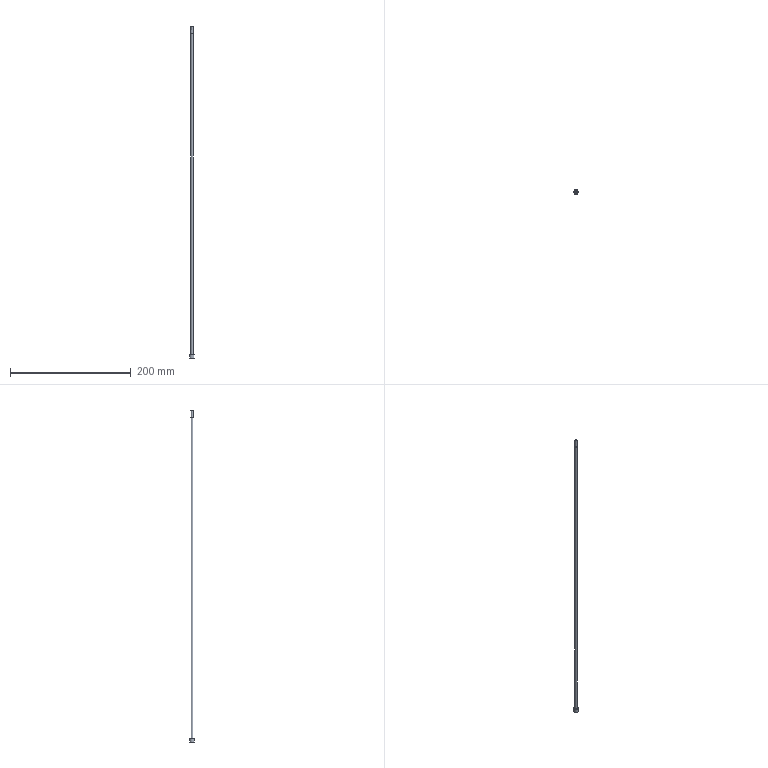Part | STEP file | solid 64 | 1 solid | 8 faces | box 8 x 8 x 549.996 mm | volume 8877 mm3 | plane 3 | cylinder 2 | torus 2 | cone 1 | commonest cylinder face diameters 4.5 x1 8 x1